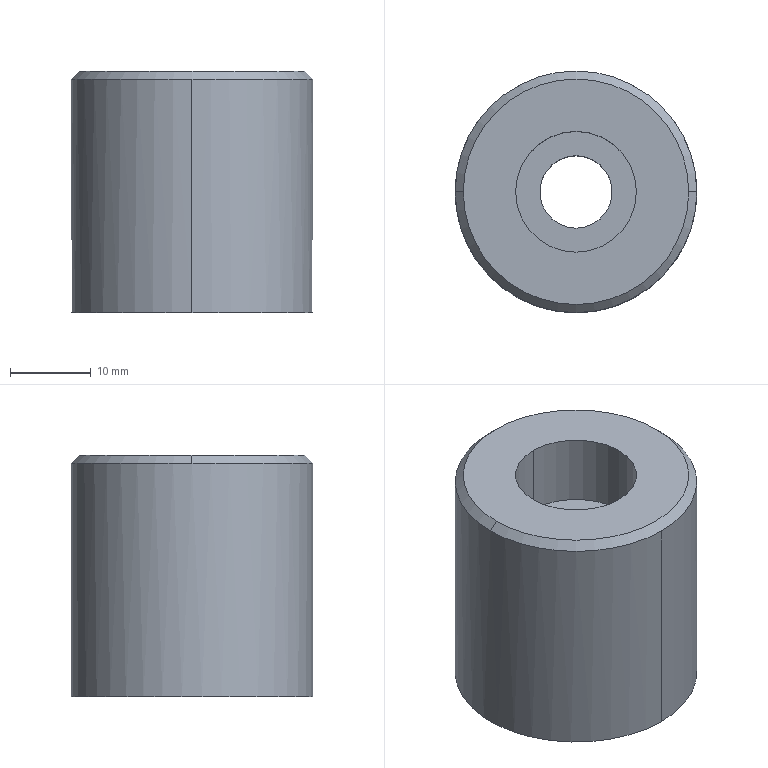Part | Creo | 1 solid | 11 faces | box 30 x 30 x 30 mm | volume 18233 mm3 | cylinder 6 | plane 3 | cone 2 | commonest cylinder face diameters 9 x2 15 x2 30 x2
STEP:
#1=CARTESIAN_POINT('',(50.,-204.505,-245.));
#2=VERTEX_POINT('',#1);
#3=CARTESIAN_POINT('',(50.,-195.505,-245.));
#4=VERTEX_POINT('',#3);
#5=CARTESIAN_POINT('',(50.,-200.005,-245.));
#6=DIRECTION('',(0.,0.,-1.));
#7=DIRECTION('',(0.,-1.,0.));
#8=AXIS2_PLACEMENT_3D('',#5,#6,#7);
#9=CIRCLE('',#8,4.5);
#10=EDGE_CURVE('',#2,#4,#9,.T.);
#11=ORIENTED_EDGE('',*,*,#10,.T.);
#12=CARTESIAN_POINT('',(50.,-195.505,-266.));
#13=VERTEX_POINT('',#12);
#14=CARTESIAN_POINT('',(50.,-195.505,-266.));
#15=DIRECTION('',(0.,0.,1.));
#16=VECTOR('',#15,21.);
#17=LINE('',#14,#16);
#18=EDGE_CURVE('',#13,#4,#17,.T.);
#19=ORIENTED_EDGE('',*,*,#18,.F.);
#20=CARTESIAN_POINT('',(50.,-204.505,-266.));
#21=VERTEX_POINT('',#20);
#22=CARTESIAN_POINT('',(50.,-200.005,-266.));
#23=DIRECTION('',(0.,0.,1.));
#24=DIRECTION('',(0.,1.,0.));
#25=AXIS2_PLACEMENT_3D('',#22,#23,#24);
#26=CIRCLE('',#25,4.5);
#27=EDGE_CURVE('',#13,#21,#26,.T.);
#28=ORIENTED_EDGE('',*,*,#27,.T.);
#29=CARTESIAN_POINT('',(50.,-204.505,-266.));
#30=DIRECTION('',(0.,0.,1.));
#31=VECTOR('',#30,21.);
#32=LINE('',#29,#31);
#33=EDGE_CURVE('',#21,#2,#32,.T.);
#34=ORIENTED_EDGE('',*,*,#33,.T.);
#35=EDGE_LOOP('',(#11,#19,#28,#34));
#36=FACE_OUTER_BOUND('',#35,.F.);
#37=CARTESIAN_POINT('',(50.,-200.005,-255.));
#38=DIRECTION('',(0.,0.,1.));
#39=DIRECTION('',(0.,1.,0.));
#40=AXIS2_PLACEMENT_3D('',#37,#38,#39);
#41=CYLINDRICAL_SURFACE('',#40,4.5);
#42=ADVANCED_FACE('',(#36),#41,.F.);
#43=CARTESIAN_POINT('',(50.,-192.505,-245.));
#44=VERTEX_POINT('',#43);
#45=CARTESIAN_POINT('',(50.,-207.505,-245.));
#46=VERTEX_POINT('',#45);
#47=CARTESIAN_POINT('',(50.,-200.005,-245.));
#48=DIRECTION('',(0.,0.,1.));
#49=DIRECTION('',(0.,1.,0.));
#50=AXIS2_PLACEMENT_3D('',#47,#48,#49);
#51=CIRCLE('',#50,7.5);
#52=EDGE_CURVE('',#44,#46,#51,.T.);
#53=ORIENTED_EDGE('',*,*,#52,.F.);
#54=CARTESIAN_POINT('',(50.,-200.005,-245.));
#55=DIRECTION('',(0.,0.,1.));
#56=DIRECTION('',(0.,-1.,0.));
#57=AXIS2_PLACEMENT_3D('',#54,#55,#56);
#58=CIRCLE('',#57,7.5);
#59=EDGE_CURVE('',#46,#44,#58,.T.);
#60=ORIENTED_EDGE('',*,*,#59,.F.);
#61=EDGE_LOOP('',(#53,#60));
#62=FACE_OUTER_BOUND('',#61,.F.);
#63=CARTESIAN_POINT('',(50.,-200.005,-245.));
#64=DIRECTION('',(0.,0.,-1.));
#65=DIRECTION('',(0.,1.,0.));
#66=AXIS2_PLACEMENT_3D('',#63,#64,#65);
#67=CIRCLE('',#66,4.5);
#68=EDGE_CURVE('',#4,#2,#67,.T.);
#69=ORIENTED_EDGE('',*,*,#68,.F.);
#70=ORIENTED_EDGE('',*,*,#10,.F.);
#71=EDGE_LOOP('',(#69,#70));
#72=FACE_BOUND('',#71,.F.);
#73=CARTESIAN_POINT('',(50.,-200.005,-245.));
#74=DIRECTION('',(0.,0.,-1.));
#75=DIRECTION('',(0.,1.,0.));
#76=AXIS2_PLACEMENT_3D('',#73,#74,#75);
#77=PLANE('',#76);
#78=ADVANCED_FACE('',(#62,#72),#77,.F.);
#79=ORIENTED_EDGE('',*,*,#68,.T.);
#80=ORIENTED_EDGE('',*,*,#33,.F.);
#81=CARTESIAN_POINT('',(50.,-200.005,-266.));
#82=DIRECTION('',(0.,0.,1.));
#83=DIRECTION('',(0.,-1.,0.));
#84=AXIS2_PLACEMENT_3D('',#81,#82,#83);
#85=CIRCLE('',#84,4.5);
#86=EDGE_CURVE('',#21,#13,#85,.T.);
#87=ORIENTED_EDGE('',*,*,#86,.T.);
#88=ORIENTED_EDGE('',*,*,#18,.T.);
#89=EDGE_LOOP('',(#79,#80,#87,#88));
#90=FACE_OUTER_BOUND('',#89,.F.);
#91=CARTESIAN_POINT('',(50.,-200.005,-255.));
#92=DIRECTION('',(0.,0.,1.));
#93=DIRECTION('',(0.,1.,0.));
#94=AXIS2_PLACEMENT_3D('',#91,#92,#93);
#95=CYLINDRICAL_SURFACE('',#94,4.5);
#96=ADVANCED_FACE('',(#90),#95,.F.);
#97=CARTESIAN_POINT('',(50.,-215.005,-266.));
#98=VERTEX_POINT('',#97);
#99=CARTESIAN_POINT('',(50.,-185.005,-266.));
#100=VERTEX_POINT('',#99);
#101=CARTESIAN_POINT('',(50.,-200.005,-266.));
#102=DIRECTION('',(0.,0.,-1.));
#103=DIRECTION('',(0.,-1.,0.));
#104=AXIS2_PLACEMENT_3D('',#101,#102,#103);
#105=CIRCLE('',#104,15.);
#106=EDGE_CURVE('',#98,#100,#105,.T.);
#107=ORIENTED_EDGE('',*,*,#106,.F.);
#108=CARTESIAN_POINT('',(50.,-200.005,-266.));
#109=DIRECTION('',(0.,0.,-1.));
#110=DIRECTION('',(0.,1.,0.));
#111=AXIS2_PLACEMENT_3D('',#108,#109,#110);
#112=CIRCLE('',#111,15.);
#113=EDGE_CURVE('',#100,#98,#112,.T.);
#114=ORIENTED_EDGE('',*,*,#113,.F.);
#115=EDGE_LOOP('',(#107,#114));
#116=FACE_OUTER_BOUND('',#115,.F.);
#117=ORIENTED_EDGE('',*,*,#27,.F.);
#118=ORIENTED_EDGE('',*,*,#86,.F.);
#119=EDGE_LOOP('',(#117,#118));
#120=FACE_BOUND('',#119,.F.);
#121=CARTESIAN_POINT('',(50.,-200.005,-266.));
#122=DIRECTION('',(0.,0.,1.));
#123=DIRECTION('',(0.,-1.,0.));
#124=AXIS2_PLACEMENT_3D('',#121,#122,#123);
#125=PLANE('',#124);
#126=ADVANCED_FACE('',(#116,#120),#125,.F.);
#127=CARTESIAN_POINT('',(35.,-200.005,-237.));
#128=VERTEX_POINT('',#127);
#129=CARTESIAN_POINT('',(50.,-215.005,-237.));
#130=VERTEX_POINT('',#129);
#131=CARTESIAN_POINT('',(50.,-200.005,-237.));
#132=DIRECTION('',(0.,0.,1.));
#133=DIRECTION('',(-1.,0.000000003,0.));
#134=AXIS2_PLACEMENT_3D('',#131,#132,#133);
#135=CIRCLE('',#134,15.);
#136=EDGE_CURVE('',#128,#130,#135,.T.);
#137=ORIENTED_EDGE('',*,*,#136,.T.);
#138=CARTESIAN_POINT('',(50.,-215.005,-266.));
#139=DIRECTION('',(0.,0.000000009,1.));
#140=VECTOR('',#139,29.);
#141=LINE('',#138,#140);
#142=EDGE_CURVE('',#98,#130,#141,.T.);
#143=ORIENTED_EDGE('',*,*,#142,.F.);
#144=ORIENTED_EDGE('',*,*,#106,.T.);
#145=CARTESIAN_POINT('',(50.,-185.005,-237.));
#146=VERTEX_POINT('',#145);
#147=CARTESIAN_POINT('',(50.,-185.005,-266.));
#148=DIRECTION('',(0.,-0.000000009,1.));
#149=VECTOR('',#148,29.);
#150=LINE('',#147,#149);
#151=EDGE_CURVE('',#100,#146,#150,.T.);
#152=ORIENTED_EDGE('',*,*,#151,.T.);
#153=CARTESIAN_POINT('',(50.,-200.005,-237.));
#154=DIRECTION('',(0.,0.,1.));
#155=DIRECTION('',(0.,1.,0.));
#156=AXIS2_PLACEMENT_3D('',#153,#154,#155);
#157=CIRCLE('',#156,15.);
#158=EDGE_CURVE('',#146,#128,#157,.T.);
#159=ORIENTED_EDGE('',*,*,#158,.T.);
#160=EDGE_LOOP('',(#137,#143,#144,#152,#159));
#161=FACE_OUTER_BOUND('',#160,.F.);
#162=CARTESIAN_POINT('',(50.,-200.005,-266.));
#163=DIRECTION('',(0.,0.,1.));
#164=DIRECTION('',(0.,-1.,0.));
#165=AXIS2_PLACEMENT_3D('',#162,#163,#164);
#166=CYLINDRICAL_SURFACE('',#165,15.);
#167=ADVANCED_FACE('',(#161),#166,.T.);
#168=CARTESIAN_POINT('',(65.,-200.005,-237.));
#169=VERTEX_POINT('',#168);
#170=CARTESIAN_POINT('',(50.,-200.005,-237.));
#171=DIRECTION('',(0.,0.,1.));
#172=DIRECTION('',(0.,-1.,0.));
#173=AXIS2_PLACEMENT_3D('',#170,#171,#172);
#174=CIRCLE('',#173,15.);
#175=EDGE_CURVE('',#130,#169,#174,.T.);
#176=ORIENTED_EDGE('',*,*,#175,.F.);
#177=ORIENTED_EDGE('',*,*,#136,.F.);
#178=CARTESIAN_POINT('',(36.,-200.005,-236.));
#179=VERTEX_POINT('',#178);
#180=CARTESIAN_POINT('',(36.,-200.005,-236.));
#181=DIRECTION('',(-0.7071,0.000000009,-0.7071));
#182=VECTOR('',#181,1.414);
#183=LINE('',#180,#182);
#184=EDGE_CURVE('',#179,#128,#183,.T.);
#185=ORIENTED_EDGE('',*,*,#184,.F.);
#186=CARTESIAN_POINT('',(50.,-214.005,-236.));
#187=VERTEX_POINT('',#186);
#188=CARTESIAN_POINT('',(50.,-200.005,-236.));
#189=DIRECTION('',(0.,0.,1.));
#190=DIRECTION('',(-1.,0.,0.));
#191=AXIS2_PLACEMENT_3D('',#188,#189,#190);
#192=CIRCLE('',#191,14.);
#193=EDGE_CURVE('',#179,#187,#192,.T.);
#194=ORIENTED_EDGE('',*,*,#193,.T.);
#195=CARTESIAN_POINT('',(64.,-200.005,-236.));
#196=VERTEX_POINT('',#195);
#197=CARTESIAN_POINT('',(50.,-200.005,-236.));
#198=DIRECTION('',(0.,0.,1.));
#199=DIRECTION('',(0.,-1.,0.));
#200=AXIS2_PLACEMENT_3D('',#197,#198,#199);
#201=CIRCLE('',#200,14.);
#202=EDGE_CURVE('',#187,#196,#201,.T.);
#203=ORIENTED_EDGE('',*,*,#202,.T.);
#204=CARTESIAN_POINT('',(64.,-200.005,-236.));
#205=DIRECTION('',(0.7071,-0.000000009,-0.7071));
#206=VECTOR('',#205,1.414);
#207=LINE('',#204,#206);
#208=EDGE_CURVE('',#196,#169,#207,.T.);
#209=ORIENTED_EDGE('',*,*,#208,.T.);
#210=EDGE_LOOP('',(#176,#177,#185,#194,#203,#209));
#211=FACE_OUTER_BOUND('',#210,.F.);
#212=CARTESIAN_POINT('',(50.,-200.005,-236.5));
#213=DIRECTION('',(0.,0.,-1.));
#214=DIRECTION('',(-1.,0.,0.));
#215=AXIS2_PLACEMENT_3D('',#212,#213,#214);
#216=CONICAL_SURFACE('',#215,14.5,45.);
#217=ADVANCED_FACE('',(#211),#216,.T.);
#218=CARTESIAN_POINT('',(50.,-200.005,-237.));
#219=DIRECTION('',(0.,0.,1.));
#220=DIRECTION('',(1.,-0.000000003,0.));
#221=AXIS2_PLACEMENT_3D('',#218,#219,#220);
#222=CIRCLE('',#221,15.);
#223=EDGE_CURVE('',#169,#146,#222,.T.);
#224=ORIENTED_EDGE('',*,*,#223,.T.);
#225=ORIENTED_EDGE('',*,*,#151,.F.);
#226=ORIENTED_EDGE('',*,*,#113,.T.);
#227=ORIENTED_EDGE('',*,*,#142,.T.);
#228=ORIENTED_EDGE('',*,*,#175,.T.);
#229=EDGE_LOOP('',(#224,#225,#226,#227,#228));
#230=FACE_OUTER_BOUND('',#229,.F.);
#231=CARTESIAN_POINT('',(50.,-200.005,-266.));
#232=DIRECTION('',(0.,0.,1.));
#233=DIRECTION('',(0.,-1.,0.));
#234=AXIS2_PLACEMENT_3D('',#231,#232,#233);
#235=CYLINDRICAL_SURFACE('',#234,15.);
#236=ADVANCED_FACE('',(#230),#235,.T.);
#237=ORIENTED_EDGE('',*,*,#223,.F.);
#238=ORIENTED_EDGE('',*,*,#208,.F.);
#239=CARTESIAN_POINT('',(50.,-186.005,-236.));
#240=VERTEX_POINT('',#239);
#241=CARTESIAN_POINT('',(50.,-200.005,-236.));
#242=DIRECTION('',(0.,0.,1.));
#243=DIRECTION('',(1.,0.,0.));
#244=AXIS2_PLACEMENT_3D('',#241,#242,#243);
#245=CIRCLE('',#244,14.);
#246=EDGE_CURVE('',#196,#240,#245,.T.);
#247=ORIENTED_EDGE('',*,*,#246,.T.);
#248=CARTESIAN_POINT('',(50.,-200.005,-236.));
#249=DIRECTION('',(0.,0.,1.));
#250=DIRECTION('',(0.,1.,0.));
#251=AXIS2_PLACEMENT_3D('',#248,#249,#250);
#252=CIRCLE('',#251,14.);
#253=EDGE_CURVE('',#240,#179,#252,.T.);
#254=ORIENTED_EDGE('',*,*,#253,.T.);
#255=ORIENTED_EDGE('',*,*,#184,.T.);
#256=ORIENTED_EDGE('',*,*,#158,.F.);
#257=EDGE_LOOP('',(#237,#238,#247,#254,#255,#256));
#258=FACE_OUTER_BOUND('',#257,.F.);
#259=CARTESIAN_POINT('',(50.,-200.005,-236.5));
#260=DIRECTION('',(0.,0.,-1.));
#261=DIRECTION('',(-1.,0.,0.));
#262=AXIS2_PLACEMENT_3D('',#259,#260,#261);
#263=CONICAL_SURFACE('',#262,14.5,45.);
#264=ADVANCED_FACE('',(#258),#263,.T.);
#265=ORIENTED_EDGE('',*,*,#202,.F.);
#266=ORIENTED_EDGE('',*,*,#193,.F.);
#267=ORIENTED_EDGE('',*,*,#253,.F.);
#268=ORIENTED_EDGE('',*,*,#246,.F.);
#269=EDGE_LOOP('',(#265,#266,#267,#268));
#270=FACE_OUTER_BOUND('',#269,.F.);
#271=CARTESIAN_POINT('',(50.,-192.505,-236.));
#272=VERTEX_POINT('',#271);
#273=CARTESIAN_POINT('',(50.,-207.505,-236.));
#274=VERTEX_POINT('',#273);
#275=CARTESIAN_POINT('',(50.,-200.005,-236.));
#276=DIRECTION('',(0.,0.,-1.));
#277=DIRECTION('',(0.,1.,0.));
#278=AXIS2_PLACEMENT_3D('',#275,#276,#277);
#279=CIRCLE('',#278,7.5);
#280=EDGE_CURVE('',#272,#274,#279,.T.);
#281=ORIENTED_EDGE('',*,*,#280,.F.);
#282=CARTESIAN_POINT('',(50.,-200.005,-236.));
#283=DIRECTION('',(0.,0.,-1.));
#284=DIRECTION('',(0.,-1.,0.));
#285=AXIS2_PLACEMENT_3D('',#282,#283,#284);
#286=CIRCLE('',#285,7.5);
#287=EDGE_CURVE('',#274,#272,#286,.T.);
#288=ORIENTED_EDGE('',*,*,#287,.F.);
#289=EDGE_LOOP('',(#281,#288));
#290=FACE_BOUND('',#289,.F.);
#291=CARTESIAN_POINT('',(50.,-200.005,-236.));
#292=DIRECTION('',(0.,0.,1.));
#293=DIRECTION('',(0.,-1.,0.));
#294=AXIS2_PLACEMENT_3D('',#291,#292,#293);
#295=PLANE('',#294);
#296=ADVANCED_FACE('',(#270,#290),#295,.T.);
#297=ORIENTED_EDGE('',*,*,#280,.T.);
#298=CARTESIAN_POINT('',(50.,-207.505,-236.));
#299=DIRECTION('',(0.,0.,-1.));
#300=VECTOR('',#299,9.);
#301=LINE('',#298,#300);
#302=EDGE_CURVE('',#274,#46,#301,.T.);
#303=ORIENTED_EDGE('',*,*,#302,.T.);
#304=ORIENTED_EDGE('',*,*,#59,.T.);
#305=CARTESIAN_POINT('',(50.,-192.505,-236.));
#306=DIRECTION('',(0.,0.,-1.));
#307=VECTOR('',#306,9.);
#308=LINE('',#305,#307);
#309=EDGE_CURVE('',#272,#44,#308,.T.);
#310=ORIENTED_EDGE('',*,*,#309,.F.);
#311=EDGE_LOOP('',(#297,#303,#304,#310));
#312=FACE_OUTER_BOUND('',#311,.F.);
#313=CARTESIAN_POINT('',(50.,-200.005,-235.55));
#314=DIRECTION('',(0.,0.,-1.));
#315=DIRECTION('',(0.,1.,0.));
#316=AXIS2_PLACEMENT_3D('',#313,#314,#315);
#317=CYLINDRICAL_SURFACE('',#316,7.5);
#318=ADVANCED_FACE('',(#312),#317,.F.);
#319=ORIENTED_EDGE('',*,*,#287,.T.);
#320=ORIENTED_EDGE('',*,*,#309,.T.);
#321=ORIENTED_EDGE('',*,*,#52,.T.);
#322=ORIENTED_EDGE('',*,*,#302,.F.);
#323=EDGE_LOOP('',(#319,#320,#321,#322));
#324=FACE_OUTER_BOUND('',#323,.F.);
#325=CARTESIAN_POINT('',(50.,-200.005,-235.55));
#326=DIRECTION('',(0.,0.,-1.));
#327=DIRECTION('',(0.,1.,0.));
#328=AXIS2_PLACEMENT_3D('',#325,#326,#327);
#329=CYLINDRICAL_SURFACE('',#328,7.5);
#330=ADVANCED_FACE('',(#324),#329,.F.);
#331=CLOSED_SHELL('',(#42,#78,#96,#126,#167,#217,#236,#264,#296,#318,#330));
#332=MANIFOLD_SOLID_BREP('',#331);
#333=(LENGTH_UNIT()NAMED_UNIT(*)SI_UNIT(.MILLI.,.METRE.));
#334=UNCERTAINTY_MEASURE_WITH_UNIT(LENGTH_MEASURE(0.005196),#333,'','');
#335=(NAMED_UNIT(*)PLANE_ANGLE_UNIT()SI_UNIT($,.RADIAN.));
#336=PLANE_ANGLE_MEASURE_WITH_UNIT(PLANE_ANGLE_MEASURE(0.01745),#335);
#337=(CONVERSION_BASED_UNIT('DEGREE',#336)NAMED_UNIT(*)PLANE_ANGLE_UNIT());
#338=(NAMED_UNIT(*)SI_UNIT($,.STERADIAN.)SOLID_ANGLE_UNIT());
#339=(GEOMETRIC_REPRESENTATION_CONTEXT(3)GLOBAL_UNCERTAINTY_ASSIGNED_CONTEXT((#334))GLOBAL_UNIT_ASSIGNED_CONTEXT((#333,#337,#338))REPRESENTATION_CONTEXT('',''));
#340=ADVANCED_BREP_SHAPE_REPRESENTATION('',(#332),#339);